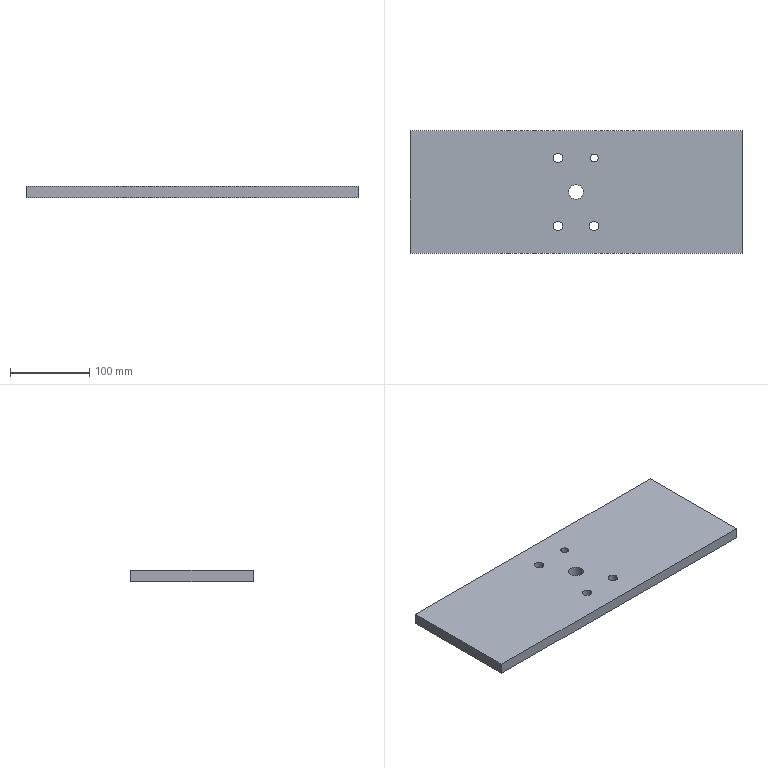Part | STEP file | Part 13^超升波生产线-2 | 1 solid | 16 faces | box 420 x 154.525 x 14 mm | volume 898915 mm3 | cylinder 10 | plane 6 | commonest cylinder face diameters 12 x4 10 x2 11.965 x2 18.715 x2
STEP:
#1=CARTESIAN_POINT('',(-9.357,0.,14.));
#2=VERTEX_POINT('',#1);
#3=CARTESIAN_POINT('',(9.357,0.,14.));
#4=VERTEX_POINT('',#3);
#5=CARTESIAN_POINT('',(0.,0.,14.));
#6=DIRECTION('',(0.,0.,1.));
#7=DIRECTION('',(1.,0.,0.));
#8=AXIS2_PLACEMENT_3D('',#5,#6,#7);
#9=CIRCLE('',#8,9.357);
#10=EDGE_CURVE('',#2,#4,#9,.T.);
#11=ORIENTED_EDGE('',*,*,#10,.T.);
#12=CARTESIAN_POINT('',(9.357,0.,0.));
#13=VERTEX_POINT('',#12);
#14=CARTESIAN_POINT('',(9.357,0.,14.));
#15=DIRECTION('',(0.,0.,-1.));
#16=VECTOR('',#15,1000.);
#17=LINE('',#14,#16);
#18=EDGE_CURVE('',#4,#13,#17,.T.);
#19=ORIENTED_EDGE('',*,*,#18,.T.);
#20=CARTESIAN_POINT('',(-9.357,0.,0.));
#21=VERTEX_POINT('',#20);
#22=CARTESIAN_POINT('',(0.,0.,0.));
#23=DIRECTION('',(0.,0.,1.));
#24=DIRECTION('',(1.,0.,0.));
#25=AXIS2_PLACEMENT_3D('',#22,#23,#24);
#26=CIRCLE('',#25,9.357);
#27=EDGE_CURVE('',#21,#13,#26,.T.);
#28=ORIENTED_EDGE('',*,*,#27,.F.);
#29=CARTESIAN_POINT('',(-9.357,0.,14.));
#30=DIRECTION('',(0.,0.,-1.));
#31=VECTOR('',#30,1000.);
#32=LINE('',#29,#31);
#33=EDGE_CURVE('',#2,#21,#32,.T.);
#34=ORIENTED_EDGE('',*,*,#33,.F.);
#35=EDGE_LOOP('',(#11,#19,#28,#34));
#36=FACE_OUTER_BOUND('',#35,.T.);
#37=CARTESIAN_POINT('',(0.,0.,14.));
#38=DIRECTION('',(0.,0.,-1.));
#39=DIRECTION('',(-1.,0.,0.));
#40=AXIS2_PLACEMENT_3D('',#37,#38,#39);
#41=CYLINDRICAL_SURFACE('',#40,9.357);
#42=ADVANCED_FACE('',(#36),#41,.F.);
#43=CARTESIAN_POINT('',(-29.,-43.,14.));
#44=VERTEX_POINT('',#43);
#45=CARTESIAN_POINT('',(-17.,-43.,14.));
#46=VERTEX_POINT('',#45);
#47=CARTESIAN_POINT('',(-23.,-43.,14.));
#48=DIRECTION('',(0.,0.,1.));
#49=DIRECTION('',(1.,0.,0.));
#50=AXIS2_PLACEMENT_3D('',#47,#48,#49);
#51=CIRCLE('',#50,6.);
#52=EDGE_CURVE('',#44,#46,#51,.T.);
#53=ORIENTED_EDGE('',*,*,#52,.T.);
#54=CARTESIAN_POINT('',(-17.,-43.,0.));
#55=VERTEX_POINT('',#54);
#56=CARTESIAN_POINT('',(-17.,-43.,14.));
#57=DIRECTION('',(0.,0.,-1.));
#58=VECTOR('',#57,1000.);
#59=LINE('',#56,#58);
#60=EDGE_CURVE('',#46,#55,#59,.T.);
#61=ORIENTED_EDGE('',*,*,#60,.T.);
#62=CARTESIAN_POINT('',(-29.,-43.,0.));
#63=VERTEX_POINT('',#62);
#64=CARTESIAN_POINT('',(-23.,-43.,0.));
#65=DIRECTION('',(0.,0.,1.));
#66=DIRECTION('',(1.,0.,0.));
#67=AXIS2_PLACEMENT_3D('',#64,#65,#66);
#68=CIRCLE('',#67,6.);
#69=EDGE_CURVE('',#63,#55,#68,.T.);
#70=ORIENTED_EDGE('',*,*,#69,.F.);
#71=CARTESIAN_POINT('',(-29.,-43.,14.));
#72=DIRECTION('',(0.,0.,-1.));
#73=VECTOR('',#72,1000.);
#74=LINE('',#71,#73);
#75=EDGE_CURVE('',#44,#63,#74,.T.);
#76=ORIENTED_EDGE('',*,*,#75,.F.);
#77=EDGE_LOOP('',(#53,#61,#70,#76));
#78=FACE_OUTER_BOUND('',#77,.T.);
#79=CARTESIAN_POINT('',(-23.,-43.,14.));
#80=DIRECTION('',(0.,0.,-1.));
#81=DIRECTION('',(-1.,0.,0.));
#82=AXIS2_PLACEMENT_3D('',#79,#80,#81);
#83=CYLINDRICAL_SURFACE('',#82,6.);
#84=ADVANCED_FACE('',(#78),#83,.F.);
#85=CARTESIAN_POINT('',(17.,-43.,14.));
#86=VERTEX_POINT('',#85);
#87=CARTESIAN_POINT('',(29.,-43.,14.));
#88=VERTEX_POINT('',#87);
#89=CARTESIAN_POINT('',(23.,-43.,14.));
#90=DIRECTION('',(0.,0.,1.));
#91=DIRECTION('',(1.,0.,0.));
#92=AXIS2_PLACEMENT_3D('',#89,#90,#91);
#93=CIRCLE('',#92,6.);
#94=EDGE_CURVE('',#86,#88,#93,.T.);
#95=ORIENTED_EDGE('',*,*,#94,.T.);
#96=CARTESIAN_POINT('',(29.,-43.,0.));
#97=VERTEX_POINT('',#96);
#98=CARTESIAN_POINT('',(29.,-43.,14.));
#99=DIRECTION('',(0.,0.,-1.));
#100=VECTOR('',#99,1000.);
#101=LINE('',#98,#100);
#102=EDGE_CURVE('',#88,#97,#101,.T.);
#103=ORIENTED_EDGE('',*,*,#102,.T.);
#104=CARTESIAN_POINT('',(17.,-43.,0.));
#105=VERTEX_POINT('',#104);
#106=CARTESIAN_POINT('',(23.,-43.,0.));
#107=DIRECTION('',(0.,0.,1.));
#108=DIRECTION('',(1.,0.,0.));
#109=AXIS2_PLACEMENT_3D('',#106,#107,#108);
#110=CIRCLE('',#109,6.);
#111=EDGE_CURVE('',#105,#97,#110,.T.);
#112=ORIENTED_EDGE('',*,*,#111,.F.);
#113=CARTESIAN_POINT('',(17.,-43.,14.));
#114=DIRECTION('',(0.,0.,-1.));
#115=VECTOR('',#114,1000.);
#116=LINE('',#113,#115);
#117=EDGE_CURVE('',#86,#105,#116,.T.);
#118=ORIENTED_EDGE('',*,*,#117,.F.);
#119=EDGE_LOOP('',(#95,#103,#112,#118));
#120=FACE_OUTER_BOUND('',#119,.T.);
#121=CARTESIAN_POINT('',(23.,-43.,14.));
#122=DIRECTION('',(0.,0.,-1.));
#123=DIRECTION('',(-1.,0.,0.));
#124=AXIS2_PLACEMENT_3D('',#121,#122,#123);
#125=CYLINDRICAL_SURFACE('',#124,6.);
#126=ADVANCED_FACE('',(#120),#125,.F.);
#127=CARTESIAN_POINT('',(-28.983,43.,14.));
#128=VERTEX_POINT('',#127);
#129=CARTESIAN_POINT('',(-17.017,43.,14.));
#130=VERTEX_POINT('',#129);
#131=CARTESIAN_POINT('',(-23.,43.,14.));
#132=DIRECTION('',(0.,0.,1.));
#133=DIRECTION('',(1.,0.,0.));
#134=AXIS2_PLACEMENT_3D('',#131,#132,#133);
#135=CIRCLE('',#134,5.983);
#136=EDGE_CURVE('',#128,#130,#135,.T.);
#137=ORIENTED_EDGE('',*,*,#136,.T.);
#138=CARTESIAN_POINT('',(-17.017,43.,0.));
#139=VERTEX_POINT('',#138);
#140=CARTESIAN_POINT('',(-17.017,43.,14.));
#141=DIRECTION('',(0.,0.,-1.));
#142=VECTOR('',#141,1000.);
#143=LINE('',#140,#142);
#144=EDGE_CURVE('',#130,#139,#143,.T.);
#145=ORIENTED_EDGE('',*,*,#144,.T.);
#146=CARTESIAN_POINT('',(-28.983,43.,0.));
#147=VERTEX_POINT('',#146);
#148=CARTESIAN_POINT('',(-23.,43.,0.));
#149=DIRECTION('',(0.,0.,1.));
#150=DIRECTION('',(1.,0.,0.));
#151=AXIS2_PLACEMENT_3D('',#148,#149,#150);
#152=CIRCLE('',#151,5.983);
#153=EDGE_CURVE('',#147,#139,#152,.T.);
#154=ORIENTED_EDGE('',*,*,#153,.F.);
#155=CARTESIAN_POINT('',(-28.983,43.,14.));
#156=DIRECTION('',(0.,0.,-1.));
#157=VECTOR('',#156,1000.);
#158=LINE('',#155,#157);
#159=EDGE_CURVE('',#128,#147,#158,.T.);
#160=ORIENTED_EDGE('',*,*,#159,.F.);
#161=EDGE_LOOP('',(#137,#145,#154,#160));
#162=FACE_OUTER_BOUND('',#161,.T.);
#163=CARTESIAN_POINT('',(-23.,43.,14.));
#164=DIRECTION('',(0.,0.,-1.));
#165=DIRECTION('',(-1.,0.,0.));
#166=AXIS2_PLACEMENT_3D('',#163,#164,#165);
#167=CYLINDRICAL_SURFACE('',#166,5.983);
#168=ADVANCED_FACE('',(#162),#167,.F.);
#169=CARTESIAN_POINT('',(18.,43.,14.));
#170=VERTEX_POINT('',#169);
#171=CARTESIAN_POINT('',(28.,43.,14.));
#172=VERTEX_POINT('',#171);
#173=CARTESIAN_POINT('',(23.,43.,14.));
#174=DIRECTION('',(0.,0.,1.));
#175=DIRECTION('',(1.,0.,0.));
#176=AXIS2_PLACEMENT_3D('',#173,#174,#175);
#177=CIRCLE('',#176,5.);
#178=EDGE_CURVE('',#170,#172,#177,.T.);
#179=ORIENTED_EDGE('',*,*,#178,.T.);
#180=CARTESIAN_POINT('',(28.,43.,0.));
#181=VERTEX_POINT('',#180);
#182=CARTESIAN_POINT('',(28.,43.,14.));
#183=DIRECTION('',(0.,0.,-1.));
#184=VECTOR('',#183,1000.);
#185=LINE('',#182,#184);
#186=EDGE_CURVE('',#172,#181,#185,.T.);
#187=ORIENTED_EDGE('',*,*,#186,.T.);
#188=CARTESIAN_POINT('',(18.,43.,0.));
#189=VERTEX_POINT('',#188);
#190=CARTESIAN_POINT('',(23.,43.,0.));
#191=DIRECTION('',(0.,0.,1.));
#192=DIRECTION('',(1.,0.,0.));
#193=AXIS2_PLACEMENT_3D('',#190,#191,#192);
#194=CIRCLE('',#193,5.);
#195=EDGE_CURVE('',#189,#181,#194,.T.);
#196=ORIENTED_EDGE('',*,*,#195,.F.);
#197=CARTESIAN_POINT('',(18.,43.,14.));
#198=DIRECTION('',(0.,0.,-1.));
#199=VECTOR('',#198,1000.);
#200=LINE('',#197,#199);
#201=EDGE_CURVE('',#170,#189,#200,.T.);
#202=ORIENTED_EDGE('',*,*,#201,.F.);
#203=EDGE_LOOP('',(#179,#187,#196,#202));
#204=FACE_OUTER_BOUND('',#203,.T.);
#205=CARTESIAN_POINT('',(23.,43.,14.));
#206=DIRECTION('',(0.,0.,-1.));
#207=DIRECTION('',(-1.,0.,0.));
#208=AXIS2_PLACEMENT_3D('',#205,#206,#207);
#209=CYLINDRICAL_SURFACE('',#208,5.);
#210=ADVANCED_FACE('',(#204),#209,.F.);
#211=ORIENTED_EDGE('',*,*,#52,.F.);
#212=CARTESIAN_POINT('',(-23.,-43.,14.));
#213=DIRECTION('',(0.,0.,1.));
#214=DIRECTION('',(1.,0.,0.));
#215=AXIS2_PLACEMENT_3D('',#212,#213,#214);
#216=CIRCLE('',#215,6.);
#217=EDGE_CURVE('',#46,#44,#216,.T.);
#218=ORIENTED_EDGE('',*,*,#217,.F.);
#219=EDGE_LOOP('',(#211,#218));
#220=FACE_BOUND('',#219,.T.);
#221=ORIENTED_EDGE('',*,*,#136,.F.);
#222=CARTESIAN_POINT('',(-23.,43.,14.));
#223=DIRECTION('',(0.,0.,1.));
#224=DIRECTION('',(1.,0.,0.));
#225=AXIS2_PLACEMENT_3D('',#222,#223,#224);
#226=CIRCLE('',#225,5.983);
#227=EDGE_CURVE('',#130,#128,#226,.T.);
#228=ORIENTED_EDGE('',*,*,#227,.F.);
#229=EDGE_LOOP('',(#221,#228));
#230=FACE_BOUND('',#229,.T.);
#231=CARTESIAN_POINT('',(210.,-77.262,14.));
#232=VERTEX_POINT('',#231);
#233=CARTESIAN_POINT('',(210.,77.262,14.));
#234=VERTEX_POINT('',#233);
#235=CARTESIAN_POINT('',(210.,-77.262,14.));
#236=DIRECTION('',(0.,1.,0.));
#237=VECTOR('',#236,1000.);
#238=LINE('',#235,#237);
#239=EDGE_CURVE('',#232,#234,#238,.T.);
#240=ORIENTED_EDGE('',*,*,#239,.T.);
#241=CARTESIAN_POINT('',(-210.,77.262,14.));
#242=VERTEX_POINT('',#241);
#243=CARTESIAN_POINT('',(-210.,77.262,14.));
#244=DIRECTION('',(-1.,0.,0.));
#245=VECTOR('',#244,1000.);
#246=LINE('',#243,#245);
#247=EDGE_CURVE('',#234,#242,#246,.T.);
#248=ORIENTED_EDGE('',*,*,#247,.T.);
#249=CARTESIAN_POINT('',(-210.,-77.262,14.));
#250=VERTEX_POINT('',#249);
#251=CARTESIAN_POINT('',(-210.,-77.262,14.));
#252=DIRECTION('',(0.,-1.,0.));
#253=VECTOR('',#252,1000.);
#254=LINE('',#251,#253);
#255=EDGE_CURVE('',#242,#250,#254,.T.);
#256=ORIENTED_EDGE('',*,*,#255,.T.);
#257=CARTESIAN_POINT('',(-210.,-77.262,14.));
#258=DIRECTION('',(1.,0.,0.));
#259=VECTOR('',#258,1000.);
#260=LINE('',#257,#259);
#261=EDGE_CURVE('',#250,#232,#260,.T.);
#262=ORIENTED_EDGE('',*,*,#261,.T.);
#263=EDGE_LOOP('',(#240,#248,#256,#262));
#264=FACE_OUTER_BOUND('',#263,.T.);
#265=ORIENTED_EDGE('',*,*,#178,.F.);
#266=CARTESIAN_POINT('',(23.,43.,14.));
#267=DIRECTION('',(0.,0.,1.));
#268=DIRECTION('',(1.,0.,0.));
#269=AXIS2_PLACEMENT_3D('',#266,#267,#268);
#270=CIRCLE('',#269,5.);
#271=EDGE_CURVE('',#172,#170,#270,.T.);
#272=ORIENTED_EDGE('',*,*,#271,.F.);
#273=EDGE_LOOP('',(#265,#272));
#274=FACE_BOUND('',#273,.T.);
#275=ORIENTED_EDGE('',*,*,#94,.F.);
#276=CARTESIAN_POINT('',(23.,-43.,14.));
#277=DIRECTION('',(0.,0.,1.));
#278=DIRECTION('',(1.,0.,0.));
#279=AXIS2_PLACEMENT_3D('',#276,#277,#278);
#280=CIRCLE('',#279,6.);
#281=EDGE_CURVE('',#88,#86,#280,.T.);
#282=ORIENTED_EDGE('',*,*,#281,.F.);
#283=EDGE_LOOP('',(#275,#282));
#284=FACE_BOUND('',#283,.T.);
#285=ORIENTED_EDGE('',*,*,#10,.F.);
#286=CARTESIAN_POINT('',(0.,0.,14.));
#287=DIRECTION('',(0.,0.,1.));
#288=DIRECTION('',(1.,0.,0.));
#289=AXIS2_PLACEMENT_3D('',#286,#287,#288);
#290=CIRCLE('',#289,9.357);
#291=EDGE_CURVE('',#4,#2,#290,.T.);
#292=ORIENTED_EDGE('',*,*,#291,.F.);
#293=EDGE_LOOP('',(#285,#292));
#294=FACE_BOUND('',#293,.T.);
#295=CARTESIAN_POINT('',(210.,77.262,14.));
#296=DIRECTION('',(0.,0.,-1.));
#297=DIRECTION('',(-1.,0.,0.));
#298=AXIS2_PLACEMENT_3D('',#295,#296,#297);
#299=PLANE('',#298);
#300=ADVANCED_FACE('',(#220,#230,#264,#274,#284,#294),#299,.F.);
#301=ORIENTED_EDGE('',*,*,#69,.T.);
#302=CARTESIAN_POINT('',(-23.,-43.,0.));
#303=DIRECTION('',(0.,0.,1.));
#304=DIRECTION('',(1.,0.,0.));
#305=AXIS2_PLACEMENT_3D('',#302,#303,#304);
#306=CIRCLE('',#305,6.);
#307=EDGE_CURVE('',#55,#63,#306,.T.);
#308=ORIENTED_EDGE('',*,*,#307,.T.);
#309=EDGE_LOOP('',(#301,#308));
#310=FACE_BOUND('',#309,.T.);
#311=ORIENTED_EDGE('',*,*,#153,.T.);
#312=CARTESIAN_POINT('',(-23.,43.,0.));
#313=DIRECTION('',(0.,0.,1.));
#314=DIRECTION('',(1.,0.,0.));
#315=AXIS2_PLACEMENT_3D('',#312,#313,#314);
#316=CIRCLE('',#315,5.983);
#317=EDGE_CURVE('',#139,#147,#316,.T.);
#318=ORIENTED_EDGE('',*,*,#317,.T.);
#319=EDGE_LOOP('',(#311,#318));
#320=FACE_BOUND('',#319,.T.);
#321=CARTESIAN_POINT('',(210.,-77.262,0.));
#322=VERTEX_POINT('',#321);
#323=CARTESIAN_POINT('',(210.,77.262,0.));
#324=VERTEX_POINT('',#323);
#325=CARTESIAN_POINT('',(210.,-77.262,0.));
#326=DIRECTION('',(0.,1.,0.));
#327=VECTOR('',#326,1000.);
#328=LINE('',#325,#327);
#329=EDGE_CURVE('',#322,#324,#328,.T.);
#330=ORIENTED_EDGE('',*,*,#329,.F.);
#331=CARTESIAN_POINT('',(-210.,-77.262,0.));
#332=VERTEX_POINT('',#331);
#333=CARTESIAN_POINT('',(-210.,-77.262,0.));
#334=DIRECTION('',(1.,0.,0.));
#335=VECTOR('',#334,1000.);
#336=LINE('',#333,#335);
#337=EDGE_CURVE('',#332,#322,#336,.T.);
#338=ORIENTED_EDGE('',*,*,#337,.F.);
#339=CARTESIAN_POINT('',(-210.,77.262,0.));
#340=VERTEX_POINT('',#339);
#341=CARTESIAN_POINT('',(-210.,-77.262,0.));
#342=DIRECTION('',(0.,-1.,0.));
#343=VECTOR('',#342,1000.);
#344=LINE('',#341,#343);
#345=EDGE_CURVE('',#340,#332,#344,.T.);
#346=ORIENTED_EDGE('',*,*,#345,.F.);
#347=CARTESIAN_POINT('',(-210.,77.262,0.));
#348=DIRECTION('',(-1.,0.,0.));
#349=VECTOR('',#348,1000.);
#350=LINE('',#347,#349);
#351=EDGE_CURVE('',#324,#340,#350,.T.);
#352=ORIENTED_EDGE('',*,*,#351,.F.);
#353=EDGE_LOOP('',(#330,#338,#346,#352));
#354=FACE_OUTER_BOUND('',#353,.T.);
#355=ORIENTED_EDGE('',*,*,#195,.T.);
#356=CARTESIAN_POINT('',(23.,43.,0.));
#357=DIRECTION('',(0.,0.,1.));
#358=DIRECTION('',(1.,0.,0.));
#359=AXIS2_PLACEMENT_3D('',#356,#357,#358);
#360=CIRCLE('',#359,5.);
#361=EDGE_CURVE('',#181,#189,#360,.T.);
#362=ORIENTED_EDGE('',*,*,#361,.T.);
#363=EDGE_LOOP('',(#355,#362));
#364=FACE_BOUND('',#363,.T.);
#365=ORIENTED_EDGE('',*,*,#111,.T.);
#366=CARTESIAN_POINT('',(23.,-43.,0.));
#367=DIRECTION('',(0.,0.,1.));
#368=DIRECTION('',(1.,0.,0.));
#369=AXIS2_PLACEMENT_3D('',#366,#367,#368);
#370=CIRCLE('',#369,6.);
#371=EDGE_CURVE('',#97,#105,#370,.T.);
#372=ORIENTED_EDGE('',*,*,#371,.T.);
#373=EDGE_LOOP('',(#365,#372));
#374=FACE_BOUND('',#373,.T.);
#375=ORIENTED_EDGE('',*,*,#27,.T.);
#376=CARTESIAN_POINT('',(0.,0.,0.));
#377=DIRECTION('',(0.,0.,1.));
#378=DIRECTION('',(1.,0.,0.));
#379=AXIS2_PLACEMENT_3D('',#376,#377,#378);
#380=CIRCLE('',#379,9.357);
#381=EDGE_CURVE('',#13,#21,#380,.T.);
#382=ORIENTED_EDGE('',*,*,#381,.T.);
#383=EDGE_LOOP('',(#375,#382));
#384=FACE_BOUND('',#383,.T.);
#385=CARTESIAN_POINT('',(210.,77.262,0.));
#386=DIRECTION('',(0.,0.,-1.));
#387=DIRECTION('',(-1.,0.,0.));
#388=AXIS2_PLACEMENT_3D('',#385,#386,#387);
#389=PLANE('',#388);
#390=ADVANCED_FACE('',(#310,#320,#354,#364,#374,#384),#389,.T.);
#391=ORIENTED_EDGE('',*,*,#329,.T.);
#392=CARTESIAN_POINT('',(210.,77.262,14.));
#393=DIRECTION('',(0.,0.,-1.));
#394=VECTOR('',#393,1000.);
#395=LINE('',#392,#394);
#396=EDGE_CURVE('',#234,#324,#395,.T.);
#397=ORIENTED_EDGE('',*,*,#396,.F.);
#398=ORIENTED_EDGE('',*,*,#239,.F.);
#399=CARTESIAN_POINT('',(210.,-77.262,14.));
#400=DIRECTION('',(0.,0.,-1.));
#401=VECTOR('',#400,1000.);
#402=LINE('',#399,#401);
#403=EDGE_CURVE('',#232,#322,#402,.T.);
#404=ORIENTED_EDGE('',*,*,#403,.T.);
#405=EDGE_LOOP('',(#391,#397,#398,#404));
#406=FACE_OUTER_BOUND('',#405,.T.);
#407=CARTESIAN_POINT('',(210.,-77.262,14.));
#408=DIRECTION('',(-1.,0.,0.));
#409=DIRECTION('',(0.,0.,1.));
#410=AXIS2_PLACEMENT_3D('',#407,#408,#409);
#411=PLANE('',#410);
#412=ADVANCED_FACE('',(#406),#411,.F.);
#413=ORIENTED_EDGE('',*,*,#351,.T.);
#414=CARTESIAN_POINT('',(-210.,77.262,14.));
#415=DIRECTION('',(0.,0.,-1.));
#416=VECTOR('',#415,1000.);
#417=LINE('',#414,#416);
#418=EDGE_CURVE('',#242,#340,#417,.T.);
#419=ORIENTED_EDGE('',*,*,#418,.F.);
#420=ORIENTED_EDGE('',*,*,#247,.F.);
#421=ORIENTED_EDGE('',*,*,#396,.T.);
#422=EDGE_LOOP('',(#413,#419,#420,#421));
#423=FACE_OUTER_BOUND('',#422,.T.);
#424=CARTESIAN_POINT('',(-210.,77.262,14.));
#425=DIRECTION('',(0.,-1.,0.));
#426=DIRECTION('',(0.,0.,-1.));
#427=AXIS2_PLACEMENT_3D('',#424,#425,#426);
#428=PLANE('',#427);
#429=ADVANCED_FACE('',(#423),#428,.F.);
#430=ORIENTED_EDGE('',*,*,#345,.T.);
#431=CARTESIAN_POINT('',(-210.,-77.262,14.));
#432=DIRECTION('',(0.,0.,-1.));
#433=VECTOR('',#432,1000.);
#434=LINE('',#431,#433);
#435=EDGE_CURVE('',#250,#332,#434,.T.);
#436=ORIENTED_EDGE('',*,*,#435,.F.);
#437=ORIENTED_EDGE('',*,*,#255,.F.);
#438=ORIENTED_EDGE('',*,*,#418,.T.);
#439=EDGE_LOOP('',(#430,#436,#437,#438));
#440=FACE_OUTER_BOUND('',#439,.T.);
#441=CARTESIAN_POINT('',(-210.,-77.262,14.));
#442=DIRECTION('',(1.,0.,0.));
#443=DIRECTION('',(0.,0.,-1.));
#444=AXIS2_PLACEMENT_3D('',#441,#442,#443);
#445=PLANE('',#444);
#446=ADVANCED_FACE('',(#440),#445,.F.);
#447=ORIENTED_EDGE('',*,*,#337,.T.);
#448=ORIENTED_EDGE('',*,*,#403,.F.);
#449=ORIENTED_EDGE('',*,*,#261,.F.);
#450=ORIENTED_EDGE('',*,*,#435,.T.);
#451=EDGE_LOOP('',(#447,#448,#449,#450));
#452=FACE_OUTER_BOUND('',#451,.T.);
#453=CARTESIAN_POINT('',(-210.,-77.262,14.));
#454=DIRECTION('',(0.,1.,0.));
#455=DIRECTION('',(0.,0.,1.));
#456=AXIS2_PLACEMENT_3D('',#453,#454,#455);
#457=PLANE('',#456);
#458=ADVANCED_FACE('',(#452),#457,.F.);
#459=ORIENTED_EDGE('',*,*,#186,.F.);
#460=ORIENTED_EDGE('',*,*,#271,.T.);
#461=ORIENTED_EDGE('',*,*,#201,.T.);
#462=ORIENTED_EDGE('',*,*,#361,.F.);
#463=EDGE_LOOP('',(#459,#460,#461,#462));
#464=FACE_OUTER_BOUND('',#463,.T.);
#465=CARTESIAN_POINT('',(23.,43.,14.));
#466=DIRECTION('',(0.,0.,-1.));
#467=DIRECTION('',(-1.,0.,0.));
#468=AXIS2_PLACEMENT_3D('',#465,#466,#467);
#469=CYLINDRICAL_SURFACE('',#468,5.);
#470=ADVANCED_FACE('',(#464),#469,.F.);
#471=ORIENTED_EDGE('',*,*,#144,.F.);
#472=ORIENTED_EDGE('',*,*,#227,.T.);
#473=ORIENTED_EDGE('',*,*,#159,.T.);
#474=ORIENTED_EDGE('',*,*,#317,.F.);
#475=EDGE_LOOP('',(#471,#472,#473,#474));
#476=FACE_OUTER_BOUND('',#475,.T.);
#477=CARTESIAN_POINT('',(-23.,43.,14.));
#478=DIRECTION('',(0.,0.,-1.));
#479=DIRECTION('',(-1.,0.,0.));
#480=AXIS2_PLACEMENT_3D('',#477,#478,#479);
#481=CYLINDRICAL_SURFACE('',#480,5.983);
#482=ADVANCED_FACE('',(#476),#481,.F.);
#483=ORIENTED_EDGE('',*,*,#102,.F.);
#484=ORIENTED_EDGE('',*,*,#281,.T.);
#485=ORIENTED_EDGE('',*,*,#117,.T.);
#486=ORIENTED_EDGE('',*,*,#371,.F.);
#487=EDGE_LOOP('',(#483,#484,#485,#486));
#488=FACE_OUTER_BOUND('',#487,.T.);
#489=CARTESIAN_POINT('',(23.,-43.,14.));
#490=DIRECTION('',(0.,0.,-1.));
#491=DIRECTION('',(-1.,0.,0.));
#492=AXIS2_PLACEMENT_3D('',#489,#490,#491);
#493=CYLINDRICAL_SURFACE('',#492,6.);
#494=ADVANCED_FACE('',(#488),#493,.F.);
#495=ORIENTED_EDGE('',*,*,#60,.F.);
#496=ORIENTED_EDGE('',*,*,#217,.T.);
#497=ORIENTED_EDGE('',*,*,#75,.T.);
#498=ORIENTED_EDGE('',*,*,#307,.F.);
#499=EDGE_LOOP('',(#495,#496,#497,#498));
#500=FACE_OUTER_BOUND('',#499,.T.);
#501=CARTESIAN_POINT('',(-23.,-43.,14.));
#502=DIRECTION('',(0.,0.,-1.));
#503=DIRECTION('',(-1.,0.,0.));
#504=AXIS2_PLACEMENT_3D('',#501,#502,#503);
#505=CYLINDRICAL_SURFACE('',#504,6.);
#506=ADVANCED_FACE('',(#500),#505,.F.);
#507=ORIENTED_EDGE('',*,*,#18,.F.);
#508=ORIENTED_EDGE('',*,*,#291,.T.);
#509=ORIENTED_EDGE('',*,*,#33,.T.);
#510=ORIENTED_EDGE('',*,*,#381,.F.);
#511=EDGE_LOOP('',(#507,#508,#509,#510));
#512=FACE_OUTER_BOUND('',#511,.T.);
#513=CARTESIAN_POINT('',(0.,0.,14.));
#514=DIRECTION('',(0.,0.,-1.));
#515=DIRECTION('',(-1.,0.,0.));
#516=AXIS2_PLACEMENT_3D('',#513,#514,#515);
#517=CYLINDRICAL_SURFACE('',#516,9.357);
#518=ADVANCED_FACE('',(#512),#517,.F.);
#519=CLOSED_SHELL('',(#42,#84,#126,#168,#210,#300,#390,#412,#429,#446,#458,#470,#482,#494,#506,#518));
#520=MANIFOLD_SOLID_BREP('',#519);
#521=CARTESIAN_POINT('',(0.,0.,0.));
#522=DIRECTION('',(0.,0.,1.));
#523=DIRECTION('',(1.,0.,0.));
#524=AXIS2_PLACEMENT_3D('',#521,#522,#523);
#525=(LENGTH_UNIT()NAMED_UNIT(*)SI_UNIT(.MILLI.,.METRE.));
#526=UNCERTAINTY_MEASURE_WITH_UNIT(LENGTH_MEASURE(0.00001),#525,'','');
#527=(NAMED_UNIT(*)PLANE_ANGLE_UNIT()SI_UNIT($,.RADIAN.));
#528=(NAMED_UNIT(*)SI_UNIT($,.STERADIAN.)SOLID_ANGLE_UNIT());
#529=(GEOMETRIC_REPRESENTATION_CONTEXT(3)GLOBAL_UNCERTAINTY_ASSIGNED_CONTEXT((#526))GLOBAL_UNIT_ASSIGNED_CONTEXT((#525,#527,#528))REPRESENTATION_CONTEXT('',''));
#530=ADVANCED_BREP_SHAPE_REPRESENTATION('',(#520,#524),#529);